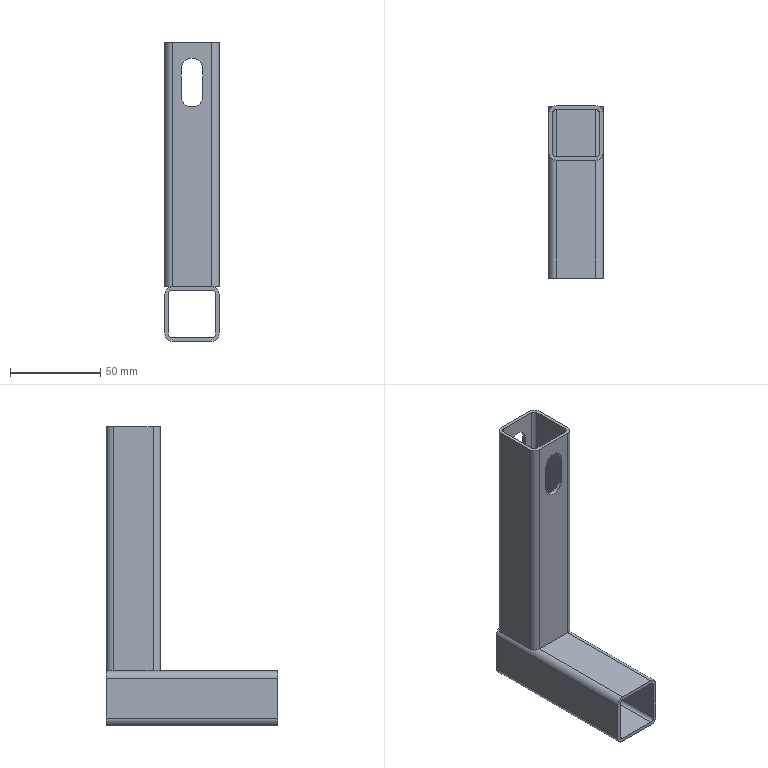Part | SolidWorks | features ICE 1, WeldMemberFeat 1, WeldmentFeature 1 | 2 solids | 46 faces | box 30 x 95 x 165 mm | volume 47978 mm3 | plane 24 | cylinder 22 | commonest cylinder face diameters 4 x8 8 x8 12 x6
STEP:
#1=CARTESIAN_POINT('',(11.,95.,15.));
#2=VERTEX_POINT('',#1);
#3=CARTESIAN_POINT('',(15.,95.,11.));
#4=VERTEX_POINT('',#3);
#5=CARTESIAN_POINT('',(11.,95.,11.));
#6=DIRECTION('',(0.,1.,0.));
#7=DIRECTION('',(0.,0.,1.));
#8=AXIS2_PLACEMENT_3D('',#5,#6,#7);
#9=CIRCLE('',#8,4.);
#10=EDGE_CURVE('',#2,#4,#9,.T.);
#11=ORIENTED_EDGE('',*,*,#10,.F.);
#12=CARTESIAN_POINT('',(11.,0.,15.));
#13=VERTEX_POINT('',#12);
#14=CARTESIAN_POINT('',(11.,80.,15.));
#15=DIRECTION('',(0.,-1.,0.));
#16=VECTOR('',#15,1000.);
#17=LINE('',#14,#16);
#18=EDGE_CURVE('',#2,#13,#17,.T.);
#19=ORIENTED_EDGE('',*,*,#18,.T.);
#20=CARTESIAN_POINT('',(15.,0.,11.));
#21=VERTEX_POINT('',#20);
#22=CARTESIAN_POINT('',(11.,0.,11.));
#23=DIRECTION('',(0.,1.,0.));
#24=DIRECTION('',(0.,0.,1.));
#25=AXIS2_PLACEMENT_3D('',#22,#23,#24);
#26=CIRCLE('',#25,4.);
#27=EDGE_CURVE('',#13,#21,#26,.T.);
#28=ORIENTED_EDGE('',*,*,#27,.T.);
#29=CARTESIAN_POINT('',(15.,80.,11.));
#30=DIRECTION('',(0.,-1.,0.));
#31=VECTOR('',#30,1000.);
#32=LINE('',#29,#31);
#33=EDGE_CURVE('',#4,#21,#32,.T.);
#34=ORIENTED_EDGE('',*,*,#33,.F.);
#35=EDGE_LOOP('',(#11,#19,#28,#34));
#36=FACE_OUTER_BOUND('',#35,.T.);
#37=CARTESIAN_POINT('',(11.,80.,11.));
#38=DIRECTION('',(0.,-1.,0.));
#39=DIRECTION('',(0.,0.,-1.));
#40=AXIS2_PLACEMENT_3D('',#37,#38,#39);
#41=CYLINDRICAL_SURFACE('',#40,4.);
#42=ADVANCED_FACE('',(#36),#41,.T.);
#43=CARTESIAN_POINT('',(15.,95.,-11.));
#44=VERTEX_POINT('',#43);
#45=CARTESIAN_POINT('',(15.,95.,11.));
#46=DIRECTION('',(0.,0.,-1.));
#47=VECTOR('',#46,1000.);
#48=LINE('',#45,#47);
#49=EDGE_CURVE('',#4,#44,#48,.T.);
#50=ORIENTED_EDGE('',*,*,#49,.F.);
#51=ORIENTED_EDGE('',*,*,#33,.T.);
#52=CARTESIAN_POINT('',(15.,0.,-11.));
#53=VERTEX_POINT('',#52);
#54=CARTESIAN_POINT('',(15.,0.,11.));
#55=DIRECTION('',(0.,0.,-1.));
#56=VECTOR('',#55,1000.);
#57=LINE('',#54,#56);
#58=EDGE_CURVE('',#21,#53,#57,.T.);
#59=ORIENTED_EDGE('',*,*,#58,.T.);
#60=CARTESIAN_POINT('',(15.,80.,-11.));
#61=DIRECTION('',(0.,-1.,0.));
#62=VECTOR('',#61,1000.);
#63=LINE('',#60,#62);
#64=EDGE_CURVE('',#44,#53,#63,.T.);
#65=ORIENTED_EDGE('',*,*,#64,.F.);
#66=EDGE_LOOP('',(#50,#51,#59,#65));
#67=FACE_OUTER_BOUND('',#66,.T.);
#68=CARTESIAN_POINT('',(15.,80.,11.));
#69=DIRECTION('',(-1.,0.,0.));
#70=DIRECTION('',(0.,0.,1.));
#71=AXIS2_PLACEMENT_3D('',#68,#69,#70);
#72=PLANE('',#71);
#73=ADVANCED_FACE('',(#67),#72,.F.);
#74=CARTESIAN_POINT('',(11.,95.,-15.));
#75=VERTEX_POINT('',#74);
#76=CARTESIAN_POINT('',(11.,95.,-11.));
#77=DIRECTION('',(0.,1.,0.));
#78=DIRECTION('',(0.,0.,1.));
#79=AXIS2_PLACEMENT_3D('',#76,#77,#78);
#80=CIRCLE('',#79,4.);
#81=EDGE_CURVE('',#44,#75,#80,.T.);
#82=ORIENTED_EDGE('',*,*,#81,.F.);
#83=ORIENTED_EDGE('',*,*,#64,.T.);
#84=CARTESIAN_POINT('',(11.,0.,-15.));
#85=VERTEX_POINT('',#84);
#86=CARTESIAN_POINT('',(11.,0.,-11.));
#87=DIRECTION('',(0.,1.,0.));
#88=DIRECTION('',(0.,0.,1.));
#89=AXIS2_PLACEMENT_3D('',#86,#87,#88);
#90=CIRCLE('',#89,4.);
#91=EDGE_CURVE('',#53,#85,#90,.T.);
#92=ORIENTED_EDGE('',*,*,#91,.T.);
#93=CARTESIAN_POINT('',(11.,80.,-15.));
#94=DIRECTION('',(0.,-1.,0.));
#95=VECTOR('',#94,1000.);
#96=LINE('',#93,#95);
#97=EDGE_CURVE('',#75,#85,#96,.T.);
#98=ORIENTED_EDGE('',*,*,#97,.F.);
#99=EDGE_LOOP('',(#82,#83,#92,#98));
#100=FACE_OUTER_BOUND('',#99,.T.);
#101=CARTESIAN_POINT('',(11.,80.,-11.));
#102=DIRECTION('',(0.,-1.,0.));
#103=DIRECTION('',(0.,0.,-1.));
#104=AXIS2_PLACEMENT_3D('',#101,#102,#103);
#105=CYLINDRICAL_SURFACE('',#104,4.);
#106=ADVANCED_FACE('',(#100),#105,.T.);
#107=CARTESIAN_POINT('',(-11.,95.,-15.));
#108=VERTEX_POINT('',#107);
#109=CARTESIAN_POINT('',(-11.,95.,-15.));
#110=DIRECTION('',(-1.,0.,0.));
#111=VECTOR('',#110,1000.);
#112=LINE('',#109,#111);
#113=EDGE_CURVE('',#75,#108,#112,.T.);
#114=ORIENTED_EDGE('',*,*,#113,.F.);
#115=ORIENTED_EDGE('',*,*,#97,.T.);
#116=CARTESIAN_POINT('',(-11.,0.,-15.));
#117=VERTEX_POINT('',#116);
#118=CARTESIAN_POINT('',(-11.,0.,-15.));
#119=DIRECTION('',(-1.,0.,0.));
#120=VECTOR('',#119,1000.);
#121=LINE('',#118,#120);
#122=EDGE_CURVE('',#85,#117,#121,.T.);
#123=ORIENTED_EDGE('',*,*,#122,.T.);
#124=CARTESIAN_POINT('',(-11.,80.,-15.));
#125=DIRECTION('',(0.,-1.,0.));
#126=VECTOR('',#125,1000.);
#127=LINE('',#124,#126);
#128=EDGE_CURVE('',#108,#117,#127,.T.);
#129=ORIENTED_EDGE('',*,*,#128,.F.);
#130=EDGE_LOOP('',(#114,#115,#123,#129));
#131=FACE_OUTER_BOUND('',#130,.T.);
#132=CARTESIAN_POINT('',(-11.,80.,-15.));
#133=DIRECTION('',(0.,0.,1.));
#134=DIRECTION('',(1.,0.,0.));
#135=AXIS2_PLACEMENT_3D('',#132,#133,#134);
#136=PLANE('',#135);
#137=ADVANCED_FACE('',(#131),#136,.F.);
#138=CARTESIAN_POINT('',(-15.,95.,-11.));
#139=VERTEX_POINT('',#138);
#140=CARTESIAN_POINT('',(-11.,95.,-11.));
#141=DIRECTION('',(0.,1.,0.));
#142=DIRECTION('',(0.,0.,1.));
#143=AXIS2_PLACEMENT_3D('',#140,#141,#142);
#144=CIRCLE('',#143,4.);
#145=EDGE_CURVE('',#108,#139,#144,.T.);
#146=ORIENTED_EDGE('',*,*,#145,.F.);
#147=ORIENTED_EDGE('',*,*,#128,.T.);
#148=CARTESIAN_POINT('',(-15.,0.,-11.));
#149=VERTEX_POINT('',#148);
#150=CARTESIAN_POINT('',(-11.,0.,-11.));
#151=DIRECTION('',(0.,1.,0.));
#152=DIRECTION('',(0.,0.,1.));
#153=AXIS2_PLACEMENT_3D('',#150,#151,#152);
#154=CIRCLE('',#153,4.);
#155=EDGE_CURVE('',#117,#149,#154,.T.);
#156=ORIENTED_EDGE('',*,*,#155,.T.);
#157=CARTESIAN_POINT('',(-15.,80.,-11.));
#158=DIRECTION('',(0.,-1.,0.));
#159=VECTOR('',#158,1000.);
#160=LINE('',#157,#159);
#161=EDGE_CURVE('',#139,#149,#160,.T.);
#162=ORIENTED_EDGE('',*,*,#161,.F.);
#163=EDGE_LOOP('',(#146,#147,#156,#162));
#164=FACE_OUTER_BOUND('',#163,.T.);
#165=CARTESIAN_POINT('',(-11.,80.,-11.));
#166=DIRECTION('',(0.,-1.,0.));
#167=DIRECTION('',(0.,0.,-1.));
#168=AXIS2_PLACEMENT_3D('',#165,#166,#167);
#169=CYLINDRICAL_SURFACE('',#168,4.);
#170=ADVANCED_FACE('',(#164),#169,.T.);
#171=CARTESIAN_POINT('',(-15.,95.,11.));
#172=VERTEX_POINT('',#171);
#173=CARTESIAN_POINT('',(-15.,95.,-11.));
#174=DIRECTION('',(0.,0.,1.));
#175=VECTOR('',#174,1000.);
#176=LINE('',#173,#175);
#177=EDGE_CURVE('',#139,#172,#176,.T.);
#178=ORIENTED_EDGE('',*,*,#177,.F.);
#179=ORIENTED_EDGE('',*,*,#161,.T.);
#180=CARTESIAN_POINT('',(-15.,0.,11.));
#181=VERTEX_POINT('',#180);
#182=CARTESIAN_POINT('',(-15.,0.,-11.));
#183=DIRECTION('',(0.,0.,1.));
#184=VECTOR('',#183,1000.);
#185=LINE('',#182,#184);
#186=EDGE_CURVE('',#149,#181,#185,.T.);
#187=ORIENTED_EDGE('',*,*,#186,.T.);
#188=CARTESIAN_POINT('',(-15.,80.,11.));
#189=DIRECTION('',(0.,-1.,0.));
#190=VECTOR('',#189,1000.);
#191=LINE('',#188,#190);
#192=EDGE_CURVE('',#172,#181,#191,.T.);
#193=ORIENTED_EDGE('',*,*,#192,.F.);
#194=EDGE_LOOP('',(#178,#179,#187,#193));
#195=FACE_OUTER_BOUND('',#194,.T.);
#196=CARTESIAN_POINT('',(-15.,80.,-11.));
#197=DIRECTION('',(1.,0.,0.));
#198=DIRECTION('',(0.,0.,-1.));
#199=AXIS2_PLACEMENT_3D('',#196,#197,#198);
#200=PLANE('',#199);
#201=ADVANCED_FACE('',(#195),#200,.F.);
#202=CARTESIAN_POINT('',(-11.,95.,15.));
#203=VERTEX_POINT('',#202);
#204=CARTESIAN_POINT('',(-11.,95.,11.));
#205=DIRECTION('',(0.,1.,0.));
#206=DIRECTION('',(0.,0.,1.));
#207=AXIS2_PLACEMENT_3D('',#204,#205,#206);
#208=CIRCLE('',#207,4.);
#209=EDGE_CURVE('',#172,#203,#208,.T.);
#210=ORIENTED_EDGE('',*,*,#209,.F.);
#211=ORIENTED_EDGE('',*,*,#192,.T.);
#212=CARTESIAN_POINT('',(-11.,0.,15.));
#213=VERTEX_POINT('',#212);
#214=CARTESIAN_POINT('',(-11.,0.,11.));
#215=DIRECTION('',(0.,1.,0.));
#216=DIRECTION('',(0.,0.,1.));
#217=AXIS2_PLACEMENT_3D('',#214,#215,#216);
#218=CIRCLE('',#217,4.);
#219=EDGE_CURVE('',#181,#213,#218,.T.);
#220=ORIENTED_EDGE('',*,*,#219,.T.);
#221=CARTESIAN_POINT('',(-11.,80.,15.));
#222=DIRECTION('',(0.,-1.,0.));
#223=VECTOR('',#222,1000.);
#224=LINE('',#221,#223);
#225=EDGE_CURVE('',#203,#213,#224,.T.);
#226=ORIENTED_EDGE('',*,*,#225,.F.);
#227=EDGE_LOOP('',(#210,#211,#220,#226));
#228=FACE_OUTER_BOUND('',#227,.T.);
#229=CARTESIAN_POINT('',(-11.,80.,11.));
#230=DIRECTION('',(0.,-1.,0.));
#231=DIRECTION('',(0.,0.,-1.));
#232=AXIS2_PLACEMENT_3D('',#229,#230,#231);
#233=CYLINDRICAL_SURFACE('',#232,4.);
#234=ADVANCED_FACE('',(#228),#233,.T.);
#235=CARTESIAN_POINT('',(13.,95.,-11.));
#236=VERTEX_POINT('',#235);
#237=CARTESIAN_POINT('',(13.,0.,-11.));
#238=VERTEX_POINT('',#237);
#239=CARTESIAN_POINT('',(13.,80.,-11.));
#240=DIRECTION('',(0.,-1.,0.));
#241=VECTOR('',#240,1000.);
#242=LINE('',#239,#241);
#243=EDGE_CURVE('',#236,#238,#242,.T.);
#244=ORIENTED_EDGE('',*,*,#243,.F.);
#245=CARTESIAN_POINT('',(11.,95.,-13.));
#246=VERTEX_POINT('',#245);
#247=CARTESIAN_POINT('',(11.,95.,-11.));
#248=DIRECTION('',(0.,1.,0.));
#249=DIRECTION('',(0.,0.,1.));
#250=AXIS2_PLACEMENT_3D('',#247,#248,#249);
#251=CIRCLE('',#250,2.);
#252=EDGE_CURVE('',#236,#246,#251,.T.);
#253=ORIENTED_EDGE('',*,*,#252,.T.);
#254=CARTESIAN_POINT('',(11.,0.,-13.));
#255=VERTEX_POINT('',#254);
#256=CARTESIAN_POINT('',(11.,80.,-13.));
#257=DIRECTION('',(0.,-1.,0.));
#258=VECTOR('',#257,1000.);
#259=LINE('',#256,#258);
#260=EDGE_CURVE('',#246,#255,#259,.T.);
#261=ORIENTED_EDGE('',*,*,#260,.T.);
#262=CARTESIAN_POINT('',(11.,0.,-11.));
#263=DIRECTION('',(0.,1.,0.));
#264=DIRECTION('',(0.,0.,1.));
#265=AXIS2_PLACEMENT_3D('',#262,#263,#264);
#266=CIRCLE('',#265,2.);
#267=EDGE_CURVE('',#238,#255,#266,.T.);
#268=ORIENTED_EDGE('',*,*,#267,.F.);
#269=EDGE_LOOP('',(#244,#253,#261,#268));
#270=FACE_OUTER_BOUND('',#269,.T.);
#271=CARTESIAN_POINT('',(11.,80.,-11.));
#272=DIRECTION('',(0.,-1.,0.));
#273=DIRECTION('',(0.,0.,-1.));
#274=AXIS2_PLACEMENT_3D('',#271,#272,#273);
#275=CYLINDRICAL_SURFACE('',#274,2.);
#276=ADVANCED_FACE('',(#270),#275,.F.);
#277=CARTESIAN_POINT('',(13.,95.,11.));
#278=VERTEX_POINT('',#277);
#279=CARTESIAN_POINT('',(13.,0.,11.));
#280=VERTEX_POINT('',#279);
#281=CARTESIAN_POINT('',(13.,80.,11.));
#282=DIRECTION('',(0.,-1.,0.));
#283=VECTOR('',#282,1000.);
#284=LINE('',#281,#283);
#285=EDGE_CURVE('',#278,#280,#284,.T.);
#286=ORIENTED_EDGE('',*,*,#285,.F.);
#287=CARTESIAN_POINT('',(13.,95.,11.));
#288=DIRECTION('',(0.,0.,-1.));
#289=VECTOR('',#288,1000.);
#290=LINE('',#287,#289);
#291=EDGE_CURVE('',#278,#236,#290,.T.);
#292=ORIENTED_EDGE('',*,*,#291,.T.);
#293=ORIENTED_EDGE('',*,*,#243,.T.);
#294=CARTESIAN_POINT('',(13.,0.,11.));
#295=DIRECTION('',(0.,0.,-1.));
#296=VECTOR('',#295,1000.);
#297=LINE('',#294,#296);
#298=EDGE_CURVE('',#280,#238,#297,.T.);
#299=ORIENTED_EDGE('',*,*,#298,.F.);
#300=EDGE_LOOP('',(#286,#292,#293,#299));
#301=FACE_OUTER_BOUND('',#300,.T.);
#302=CARTESIAN_POINT('',(13.,80.,11.));
#303=DIRECTION('',(-1.,0.,0.));
#304=DIRECTION('',(0.,0.,1.));
#305=AXIS2_PLACEMENT_3D('',#302,#303,#304);
#306=PLANE('',#305);
#307=ADVANCED_FACE('',(#301),#306,.T.);
#308=CARTESIAN_POINT('',(11.,95.,13.));
#309=VERTEX_POINT('',#308);
#310=CARTESIAN_POINT('',(11.,0.,13.));
#311=VERTEX_POINT('',#310);
#312=CARTESIAN_POINT('',(11.,80.,13.));
#313=DIRECTION('',(0.,-1.,0.));
#314=VECTOR('',#313,1000.);
#315=LINE('',#312,#314);
#316=EDGE_CURVE('',#309,#311,#315,.T.);
#317=ORIENTED_EDGE('',*,*,#316,.F.);
#318=CARTESIAN_POINT('',(11.,95.,11.));
#319=DIRECTION('',(0.,1.,0.));
#320=DIRECTION('',(0.,0.,1.));
#321=AXIS2_PLACEMENT_3D('',#318,#319,#320);
#322=CIRCLE('',#321,2.);
#323=EDGE_CURVE('',#309,#278,#322,.T.);
#324=ORIENTED_EDGE('',*,*,#323,.T.);
#325=ORIENTED_EDGE('',*,*,#285,.T.);
#326=CARTESIAN_POINT('',(11.,0.,11.));
#327=DIRECTION('',(0.,1.,0.));
#328=DIRECTION('',(0.,0.,1.));
#329=AXIS2_PLACEMENT_3D('',#326,#327,#328);
#330=CIRCLE('',#329,2.);
#331=EDGE_CURVE('',#311,#280,#330,.T.);
#332=ORIENTED_EDGE('',*,*,#331,.F.);
#333=EDGE_LOOP('',(#317,#324,#325,#332));
#334=FACE_OUTER_BOUND('',#333,.T.);
#335=CARTESIAN_POINT('',(11.,80.,11.));
#336=DIRECTION('',(0.,-1.,0.));
#337=DIRECTION('',(0.,0.,-1.));
#338=AXIS2_PLACEMENT_3D('',#335,#336,#337);
#339=CYLINDRICAL_SURFACE('',#338,2.);
#340=ADVANCED_FACE('',(#334),#339,.F.);
#341=CARTESIAN_POINT('',(-11.,95.,13.));
#342=VERTEX_POINT('',#341);
#343=CARTESIAN_POINT('',(-11.,0.,13.));
#344=VERTEX_POINT('',#343);
#345=CARTESIAN_POINT('',(-11.,80.,13.));
#346=DIRECTION('',(0.,-1.,0.));
#347=VECTOR('',#346,1000.);
#348=LINE('',#345,#347);
#349=EDGE_CURVE('',#342,#344,#348,.T.);
#350=ORIENTED_EDGE('',*,*,#349,.F.);
#351=CARTESIAN_POINT('',(11.,95.,13.));
#352=DIRECTION('',(1.,0.,0.));
#353=VECTOR('',#352,1000.);
#354=LINE('',#351,#353);
#355=EDGE_CURVE('',#342,#309,#354,.T.);
#356=ORIENTED_EDGE('',*,*,#355,.T.);
#357=ORIENTED_EDGE('',*,*,#316,.T.);
#358=CARTESIAN_POINT('',(11.,0.,13.));
#359=DIRECTION('',(1.,0.,0.));
#360=VECTOR('',#359,1000.);
#361=LINE('',#358,#360);
#362=EDGE_CURVE('',#344,#311,#361,.T.);
#363=ORIENTED_EDGE('',*,*,#362,.F.);
#364=EDGE_LOOP('',(#350,#356,#357,#363));
#365=FACE_OUTER_BOUND('',#364,.T.);
#366=CARTESIAN_POINT('',(11.,80.,13.));
#367=DIRECTION('',(0.,0.,-1.));
#368=DIRECTION('',(-1.,0.,0.));
#369=AXIS2_PLACEMENT_3D('',#366,#367,#368);
#370=PLANE('',#369);
#371=ADVANCED_FACE('',(#365),#370,.T.);
#372=CARTESIAN_POINT('',(-13.,95.,11.));
#373=VERTEX_POINT('',#372);
#374=CARTESIAN_POINT('',(-13.,0.,11.));
#375=VERTEX_POINT('',#374);
#376=CARTESIAN_POINT('',(-13.,80.,11.));
#377=DIRECTION('',(0.,-1.,0.));
#378=VECTOR('',#377,1000.);
#379=LINE('',#376,#378);
#380=EDGE_CURVE('',#373,#375,#379,.T.);
#381=ORIENTED_EDGE('',*,*,#380,.F.);
#382=CARTESIAN_POINT('',(-11.,95.,11.));
#383=DIRECTION('',(0.,1.,0.));
#384=DIRECTION('',(0.,0.,1.));
#385=AXIS2_PLACEMENT_3D('',#382,#383,#384);
#386=CIRCLE('',#385,2.);
#387=EDGE_CURVE('',#373,#342,#386,.T.);
#388=ORIENTED_EDGE('',*,*,#387,.T.);
#389=ORIENTED_EDGE('',*,*,#349,.T.);
#390=CARTESIAN_POINT('',(-11.,0.,11.));
#391=DIRECTION('',(0.,1.,0.));
#392=DIRECTION('',(0.,0.,1.));
#393=AXIS2_PLACEMENT_3D('',#390,#391,#392);
#394=CIRCLE('',#393,2.);
#395=EDGE_CURVE('',#375,#344,#394,.T.);
#396=ORIENTED_EDGE('',*,*,#395,.F.);
#397=EDGE_LOOP('',(#381,#388,#389,#396));
#398=FACE_OUTER_BOUND('',#397,.T.);
#399=CARTESIAN_POINT('',(-11.,80.,11.));
#400=DIRECTION('',(0.,-1.,0.));
#401=DIRECTION('',(0.,0.,-1.));
#402=AXIS2_PLACEMENT_3D('',#399,#400,#401);
#403=CYLINDRICAL_SURFACE('',#402,2.);
#404=ADVANCED_FACE('',(#398),#403,.F.);
#405=CARTESIAN_POINT('',(-13.,95.,-11.));
#406=VERTEX_POINT('',#405);
#407=CARTESIAN_POINT('',(-13.,0.,-11.));
#408=VERTEX_POINT('',#407);
#409=CARTESIAN_POINT('',(-13.,80.,-11.));
#410=DIRECTION('',(0.,-1.,0.));
#411=VECTOR('',#410,1000.);
#412=LINE('',#409,#411);
#413=EDGE_CURVE('',#406,#408,#412,.T.);
#414=ORIENTED_EDGE('',*,*,#413,.F.);
#415=CARTESIAN_POINT('',(-13.,95.,-11.));
#416=DIRECTION('',(0.,0.,1.));
#417=VECTOR('',#416,1000.);
#418=LINE('',#415,#417);
#419=EDGE_CURVE('',#406,#373,#418,.T.);
#420=ORIENTED_EDGE('',*,*,#419,.T.);
#421=ORIENTED_EDGE('',*,*,#380,.T.);
#422=CARTESIAN_POINT('',(-13.,0.,-11.));
#423=DIRECTION('',(0.,0.,1.));
#424=VECTOR('',#423,1000.);
#425=LINE('',#422,#424);
#426=EDGE_CURVE('',#408,#375,#425,.T.);
#427=ORIENTED_EDGE('',*,*,#426,.F.);
#428=EDGE_LOOP('',(#414,#420,#421,#427));
#429=FACE_OUTER_BOUND('',#428,.T.);
#430=CARTESIAN_POINT('',(-13.,80.,-11.));
#431=DIRECTION('',(1.,0.,0.));
#432=DIRECTION('',(0.,0.,-1.));
#433=AXIS2_PLACEMENT_3D('',#430,#431,#432);
#434=PLANE('',#433);
#435=ADVANCED_FACE('',(#429),#434,.T.);
#436=CARTESIAN_POINT('',(-11.,95.,-13.));
#437=VERTEX_POINT('',#436);
#438=CARTESIAN_POINT('',(-11.,0.,-13.));
#439=VERTEX_POINT('',#438);
#440=CARTESIAN_POINT('',(-11.,80.,-13.));
#441=DIRECTION('',(0.,-1.,0.));
#442=VECTOR('',#441,1000.);
#443=LINE('',#440,#442);
#444=EDGE_CURVE('',#437,#439,#443,.T.);
#445=ORIENTED_EDGE('',*,*,#444,.F.);
#446=CARTESIAN_POINT('',(-11.,95.,-11.));
#447=DIRECTION('',(0.,1.,0.));
#448=DIRECTION('',(0.,0.,1.));
#449=AXIS2_PLACEMENT_3D('',#446,#447,#448);
#450=CIRCLE('',#449,2.);
#451=EDGE_CURVE('',#437,#406,#450,.T.);
#452=ORIENTED_EDGE('',*,*,#451,.T.);
#453=ORIENTED_EDGE('',*,*,#413,.T.);
#454=CARTESIAN_POINT('',(-11.,0.,-11.));
#455=DIRECTION('',(0.,1.,0.));
#456=DIRECTION('',(0.,0.,1.));
#457=AXIS2_PLACEMENT_3D('',#454,#455,#456);
#458=CIRCLE('',#457,2.);
#459=EDGE_CURVE('',#439,#408,#458,.T.);
#460=ORIENTED_EDGE('',*,*,#459,.F.);
#461=EDGE_LOOP('',(#445,#452,#453,#460));
#462=FACE_OUTER_BOUND('',#461,.T.);
#463=CARTESIAN_POINT('',(-11.,80.,-11.));
#464=DIRECTION('',(0.,-1.,0.));
#465=DIRECTION('',(0.,0.,-1.));
#466=AXIS2_PLACEMENT_3D('',#463,#464,#465);
#467=CYLINDRICAL_SURFACE('',#466,2.);
#468=ADVANCED_FACE('',(#462),#467,.F.);
#469=ORIENTED_EDGE('',*,*,#260,.F.);
#470=CARTESIAN_POINT('',(-11.,95.,-13.));
#471=DIRECTION('',(-1.,0.,0.));
#472=VECTOR('',#471,1000.);
#473=LINE('',#470,#472);
#474=EDGE_CURVE('',#246,#437,#473,.T.);
#475=ORIENTED_EDGE('',*,*,#474,.T.);
#476=ORIENTED_EDGE('',*,*,#444,.T.);
#477=CARTESIAN_POINT('',(-11.,0.,-13.));
#478=DIRECTION('',(-1.,0.,0.));
#479=VECTOR('',#478,1000.);
#480=LINE('',#477,#479);
#481=EDGE_CURVE('',#255,#439,#480,.T.);
#482=ORIENTED_EDGE('',*,*,#481,.F.);
#483=EDGE_LOOP('',(#469,#475,#476,#482));
#484=FACE_OUTER_BOUND('',#483,.T.);
#485=CARTESIAN_POINT('',(-11.,80.,-13.));
#486=DIRECTION('',(0.,0.,1.));
#487=DIRECTION('',(1.,0.,0.));
#488=AXIS2_PLACEMENT_3D('',#485,#486,#487);
#489=PLANE('',#488);
#490=ADVANCED_FACE('',(#484),#489,.T.);
#491=CARTESIAN_POINT('',(11.,95.,15.));
#492=DIRECTION('',(1.,0.,0.));
#493=VECTOR('',#492,1000.);
#494=LINE('',#491,#493);
#495=EDGE_CURVE('',#203,#2,#494,.T.);
#496=ORIENTED_EDGE('',*,*,#495,.F.);
#497=ORIENTED_EDGE('',*,*,#225,.T.);
#498=CARTESIAN_POINT('',(11.,0.,15.));
#499=DIRECTION('',(1.,0.,0.));
#500=VECTOR('',#499,1000.);
#501=LINE('',#498,#500);
#502=EDGE_CURVE('',#213,#13,#501,.T.);
#503=ORIENTED_EDGE('',*,*,#502,.T.);
#504=ORIENTED_EDGE('',*,*,#18,.F.);
#505=EDGE_LOOP('',(#496,#497,#503,#504));
#506=FACE_OUTER_BOUND('',#505,.T.);
#507=CARTESIAN_POINT('',(11.,80.,15.));
#508=DIRECTION('',(0.,0.,-1.));
#509=DIRECTION('',(-1.,0.,0.));
#510=AXIS2_PLACEMENT_3D('',#507,#508,#509);
#511=PLANE('',#510);
#512=ADVANCED_FACE('',(#506),#511,.F.);
#513=ORIENTED_EDGE('',*,*,#267,.T.);
#514=ORIENTED_EDGE('',*,*,#481,.T.);
#515=ORIENTED_EDGE('',*,*,#459,.T.);
#516=ORIENTED_EDGE('',*,*,#426,.T.);
#517=ORIENTED_EDGE('',*,*,#395,.T.);
#518=ORIENTED_EDGE('',*,*,#362,.T.);
#519=ORIENTED_EDGE('',*,*,#331,.T.);
#520=ORIENTED_EDGE('',*,*,#298,.T.);
#521=EDGE_LOOP('',(#513,#514,#515,#516,#517,#518,#519,#520));
#522=FACE_BOUND('',#521,.T.);
#523=ORIENTED_EDGE('',*,*,#27,.F.);
#524=ORIENTED_EDGE('',*,*,#502,.F.);
#525=ORIENTED_EDGE('',*,*,#219,.F.);
#526=ORIENTED_EDGE('',*,*,#186,.F.);
#527=ORIENTED_EDGE('',*,*,#155,.F.);
#528=ORIENTED_EDGE('',*,*,#122,.F.);
#529=ORIENTED_EDGE('',*,*,#91,.F.);
#530=ORIENTED_EDGE('',*,*,#58,.F.);
#531=EDGE_LOOP('',(#523,#524,#525,#526,#527,#528,#529,#530));
#532=FACE_OUTER_BOUND('',#531,.T.);
#533=CARTESIAN_POINT('',(11.,0.,11.));
#534=DIRECTION('',(0.,1.,0.));
#535=DIRECTION('',(0.,0.,1.));
#536=AXIS2_PLACEMENT_3D('',#533,#534,#535);
#537=PLANE('',#536);
#538=ADVANCED_FACE('',(#522,#532),#537,.F.);
#539=ORIENTED_EDGE('',*,*,#252,.F.);
#540=ORIENTED_EDGE('',*,*,#291,.F.);
#541=ORIENTED_EDGE('',*,*,#323,.F.);
#542=ORIENTED_EDGE('',*,*,#355,.F.);
#543=ORIENTED_EDGE('',*,*,#387,.F.);
#544=ORIENTED_EDGE('',*,*,#419,.F.);
#545=ORIENTED_EDGE('',*,*,#451,.F.);
#546=ORIENTED_EDGE('',*,*,#474,.F.);
#547=EDGE_LOOP('',(#539,#540,#541,#542,#543,#544,#545,#546));
#548=FACE_BOUND('',#547,.T.);
#549=ORIENTED_EDGE('',*,*,#495,.T.);
#550=ORIENTED_EDGE('',*,*,#10,.T.);
#551=ORIENTED_EDGE('',*,*,#49,.T.);
#552=ORIENTED_EDGE('',*,*,#81,.T.);
#553=ORIENTED_EDGE('',*,*,#113,.T.);
#554=ORIENTED_EDGE('',*,*,#145,.T.);
#555=ORIENTED_EDGE('',*,*,#177,.T.);
#556=ORIENTED_EDGE('',*,*,#209,.T.);
#557=EDGE_LOOP('',(#549,#550,#551,#552,#553,#554,#555,#556));
#558=FACE_OUTER_BOUND('',#557,.T.);
#559=CARTESIAN_POINT('',(15.,95.,0.));
#560=DIRECTION('',(0.,1.,0.));
#561=DIRECTION('',(0.,0.,1.));
#562=AXIS2_PLACEMENT_3D('',#559,#560,#561);
#563=PLANE('',#562);
#564=ADVANCED_FACE('',(#548,#558),#563,.T.);
#565=CLOSED_SHELL('',(#42,#73,#106,#137,#170,#201,#234,#276,#307,#340,#371,#404,#435,#468,#490,#512,#538,#564));
#566=MANIFOLD_SOLID_BREP('',#565);
#567=CARTESIAN_POINT('',(6.,93.,135.514));
#568=VERTEX_POINT('',#567);
#569=CARTESIAN_POINT('',(0.,93.,141.514));
#570=VERTEX_POINT('',#569);
#571=CARTESIAN_POINT('',(0.,93.,135.514));
#572=DIRECTION('',(0.,-1.,0.));
#573=DIRECTION('',(0.,0.,-1.));
#574=AXIS2_PLACEMENT_3D('',#571,#572,#573);
#575=CIRCLE('',#574,6.);
#576=EDGE_CURVE('',#568,#570,#575,.T.);
#577=ORIENTED_EDGE('',*,*,#576,.T.);
#578=CARTESIAN_POINT('',(0.,95.,141.514));
#579=VERTEX_POINT('',#578);
#580=CARTESIAN_POINT('',(0.,28.,141.514));
#581=DIRECTION('',(0.,1.,0.));
#582=VECTOR('',#581,1000.);
#583=LINE('',#580,#582);
#584=EDGE_CURVE('',#570,#579,#583,.T.);
#585=ORIENTED_EDGE('',*,*,#584,.T.);
#586=CARTESIAN_POINT('',(6.,95.,135.514));
#587=VERTEX_POINT('',#586);
#588=CARTESIAN_POINT('',(0.,95.,135.514));
#589=DIRECTION('',(0.,1.,0.));
#590=DIRECTION('',(0.,0.,1.));
#591=AXIS2_PLACEMENT_3D('',#588,#589,#590);
#592=CIRCLE('',#591,6.);
#593=EDGE_CURVE('',#579,#587,#592,.T.);
#594=ORIENTED_EDGE('',*,*,#593,.T.);
#595=CARTESIAN_POINT('',(6.,28.,135.514));
#596=DIRECTION('',(0.,1.,0.));
#597=VECTOR('',#596,1000.);
#598=LINE('',#595,#597);
#599=EDGE_CURVE('',#568,#587,#598,.T.);
#600=ORIENTED_EDGE('',*,*,#599,.F.);
#601=EDGE_LOOP('',(#577,#585,#594,#600));
#602=FACE_OUTER_BOUND('',#601,.T.);
#603=CARTESIAN_POINT('',(0.,28.,135.514));
#604=DIRECTION('',(0.,1.,0.));
#605=DIRECTION('',(0.,0.,1.));
#606=AXIS2_PLACEMENT_3D('',#603,#604,#605);
#607=CYLINDRICAL_SURFACE('',#606,6.);
#608=ADVANCED_FACE('',(#602),#607,.F.);
#609=CARTESIAN_POINT('',(0.,65.,141.514));
#610=VERTEX_POINT('',#609);
#611=CARTESIAN_POINT('',(6.,65.,135.514));
#612=VERTEX_POINT('',#611);
#613=CARTESIAN_POINT('',(0.,65.,135.514));
#614=DIRECTION('',(0.,1.,0.));
#615=DIRECTION('',(0.,0.,1.));
#616=AXIS2_PLACEMENT_3D('',#613,#614,#615);
#617=CIRCLE('',#616,6.);
#618=EDGE_CURVE('',#610,#612,#617,.T.);
#619=ORIENTED_EDGE('',*,*,#618,.F.);
#620=CARTESIAN_POINT('',(0.,67.,141.514));
#621=VERTEX_POINT('',#620);
#622=CARTESIAN_POINT('',(0.,28.,141.514));
#623=DIRECTION('',(0.,1.,0.));
#624=VECTOR('',#623,1000.);
#625=LINE('',#622,#624);
#626=EDGE_CURVE('',#610,#621,#625,.T.);
#627=ORIENTED_EDGE('',*,*,#626,.T.);
#628=CARTESIAN_POINT('',(6.,67.,135.514));
#629=VERTEX_POINT('',#628);
#630=CARTESIAN_POINT('',(0.,67.,135.514));
#631=DIRECTION('',(0.,1.,0.));
#632=DIRECTION('',(0.,0.,1.));
#633=AXIS2_PLACEMENT_3D('',#630,#631,#632);
#634=CIRCLE('',#633,6.);
#635=EDGE_CURVE('',#621,#629,#634,.T.);
#636=ORIENTED_EDGE('',*,*,#635,.T.);
#637=CARTESIAN_POINT('',(6.,28.,135.514));
#638=DIRECTION('',(0.,1.,0.));
#639=VECTOR('',#638,1000.);
#640=LINE('',#637,#639);
#641=EDGE_CURVE('',#612,#629,#640,.T.);
#642=ORIENTED_EDGE('',*,*,#641,.F.);
#643=EDGE_LOOP('',(#619,#627,#636,#642));
#644=FACE_OUTER_BOUND('',#643,.T.);
#645=CARTESIAN_POINT('',(0.,28.,135.514));
#646=DIRECTION('',(0.,1.,0.));
#647=DIRECTION('',(0.,0.,1.));
#648=AXIS2_PLACEMENT_3D('',#645,#646,#647);
#649=CYLINDRICAL_SURFACE('',#648,6.);
#650=ADVANCED_FACE('',(#644),#649,.F.);
#651=CARTESIAN_POINT('',(15.,69.,15.));
#652=VERTEX_POINT('',#651);
#653=CARTESIAN_POINT('',(11.,65.,15.));
#654=VERTEX_POINT('',#653);
#655=CARTESIAN_POINT('',(11.,69.,15.));
#656=DIRECTION('',(0.,0.,-1.));
#657=DIRECTION('',(-1.,0.,0.));
#658=AXIS2_PLACEMENT_3D('',#655,#656,#657);
#659=CIRCLE('',#658,4.);
#660=EDGE_CURVE('',#652,#654,#659,.T.);
#661=ORIENTED_EDGE('',*,*,#660,.F.);
#662=CARTESIAN_POINT('',(15.,69.,150.));
#663=VERTEX_POINT('',#662);
#664=CARTESIAN_POINT('',(15.,69.,150.));
#665=DIRECTION('',(0.,0.,-1.));
#666=VECTOR('',#665,1000.);
#667=LINE('',#664,#666);
#668=EDGE_CURVE('',#663,#652,#667,.T.);
#669=ORIENTED_EDGE('',*,*,#668,.F.);
#670=CARTESIAN_POINT('',(11.,65.,150.));
#671=VERTEX_POINT('',#670);
#672=CARTESIAN_POINT('',(11.,69.,150.));
#673=DIRECTION('',(0.,0.,1.));
#674=DIRECTION('',(0.,-1.,0.));
#675=AXIS2_PLACEMENT_3D('',#672,#673,#674);
#676=CIRCLE('',#675,4.);
#677=EDGE_CURVE('',#671,#663,#676,.T.);
#678=ORIENTED_EDGE('',*,*,#677,.F.);
#679=CARTESIAN_POINT('',(11.,65.,150.));
#680=DIRECTION('',(0.,0.,-1.));
#681=VECTOR('',#680,1000.);
#682=LINE('',#679,#681);
#683=EDGE_CURVE('',#671,#654,#682,.T.);
#684=ORIENTED_EDGE('',*,*,#683,.T.);
#685=EDGE_LOOP('',(#661,#669,#678,#684));
#686=FACE_OUTER_BOUND('',#685,.T.);
#687=CARTESIAN_POINT('',(11.,69.,150.));
#688=DIRECTION('',(0.,0.,-1.));
#689=DIRECTION('',(0.,1.,0.));
#690=AXIS2_PLACEMENT_3D('',#687,#688,#689);
#691=CYLINDRICAL_SURFACE('',#690,4.);
#692=ADVANCED_FACE('',(#686),#691,.T.);
#693=CARTESIAN_POINT('',(15.,91.,15.));
#694=VERTEX_POINT('',#693);
#695=CARTESIAN_POINT('',(15.,80.,15.));
#696=DIRECTION('',(0.,-1.,0.));
#697=VECTOR('',#696,1000.);
#698=LINE('',#695,#697);
#699=EDGE_CURVE('',#694,#652,#698,.T.);
#700=ORIENTED_EDGE('',*,*,#699,.F.);
#701=CARTESIAN_POINT('',(15.,91.,150.));
#702=VERTEX_POINT('',#701);
#703=CARTESIAN_POINT('',(15.,91.,150.));
#704=DIRECTION('',(0.,0.,-1.));
#705=VECTOR('',#704,1000.);
#706=LINE('',#703,#705);
#707=EDGE_CURVE('',#702,#694,#706,.T.);
#708=ORIENTED_EDGE('',*,*,#707,.F.);
#709=CARTESIAN_POINT('',(15.,69.,150.));
#710=DIRECTION('',(0.,1.,0.));
#711=VECTOR('',#710,1000.);
#712=LINE('',#709,#711);
#713=EDGE_CURVE('',#663,#702,#712,.T.);
#714=ORIENTED_EDGE('',*,*,#713,.F.);
#715=ORIENTED_EDGE('',*,*,#668,.T.);
#716=EDGE_LOOP('',(#700,#708,#714,#715));
#717=FACE_OUTER_BOUND('',#716,.T.);
#718=CARTESIAN_POINT('',(15.,69.,150.));
#719=DIRECTION('',(-1.,0.,0.));
#720=DIRECTION('',(0.,0.,1.));
#721=AXIS2_PLACEMENT_3D('',#718,#719,#720);
#722=PLANE('',#721);
#723=ADVANCED_FACE('',(#717),#722,.F.);
#724=CARTESIAN_POINT('',(11.,95.,15.));
#725=VERTEX_POINT('',#724);
#726=CARTESIAN_POINT('',(11.,91.,15.));
#727=DIRECTION('',(0.,0.,-1.));
#728=DIRECTION('',(-1.,0.,0.));
#729=AXIS2_PLACEMENT_3D('',#726,#727,#728);
#730=CIRCLE('',#729,4.);
#731=EDGE_CURVE('',#725,#694,#730,.T.);
#732=ORIENTED_EDGE('',*,*,#731,.F.);
#733=CARTESIAN_POINT('',(11.,95.,150.));
#734=VERTEX_POINT('',#733);
#735=CARTESIAN_POINT('',(11.,95.,150.));
#736=DIRECTION('',(0.,0.,-1.));
#737=VECTOR('',#736,1000.);
#738=LINE('',#735,#737);
#739=EDGE_CURVE('',#734,#725,#738,.T.);
#740=ORIENTED_EDGE('',*,*,#739,.F.);
#741=CARTESIAN_POINT('',(11.,91.,150.));
#742=DIRECTION('',(0.,0.,1.));
#743=DIRECTION('',(0.,-1.,0.));
#744=AXIS2_PLACEMENT_3D('',#741,#742,#743);
#745=CIRCLE('',#744,4.);
#746=EDGE_CURVE('',#702,#734,#745,.T.);
#747=ORIENTED_EDGE('',*,*,#746,.F.);
#748=ORIENTED_EDGE('',*,*,#707,.T.);
#749=EDGE_LOOP('',(#732,#740,#747,#748));
#750=FACE_OUTER_BOUND('',#749,.T.);
#751=CARTESIAN_POINT('',(11.,91.,150.));
#752=DIRECTION('',(0.,0.,-1.));
#753=DIRECTION('',(0.,1.,0.));
#754=AXIS2_PLACEMENT_3D('',#751,#752,#753);
#755=CYLINDRICAL_SURFACE('',#754,4.);
#756=ADVANCED_FACE('',(#750),#755,.T.);
#757=CARTESIAN_POINT('',(6.,95.,120.514));
#758=VERTEX_POINT('',#757);
#759=CARTESIAN_POINT('',(6.,95.,135.514));
#760=DIRECTION('',(0.,0.,-1.));
#761=VECTOR('',#760,1000.);
#762=LINE('',#759,#761);
#763=EDGE_CURVE('',#587,#758,#762,.T.);
#764=ORIENTED_EDGE('',*,*,#763,.F.);
#765=ORIENTED_EDGE('',*,*,#593,.F.);
#766=CARTESIAN_POINT('',(-6.,95.,135.514));
#767=VERTEX_POINT('',#766);
#768=CARTESIAN_POINT('',(0.,95.,135.514));
#769=DIRECTION('',(0.,1.,0.));
#770=DIRECTION('',(0.,0.,1.));
#771=AXIS2_PLACEMENT_3D('',#768,#769,#770);
#772=CIRCLE('',#771,6.);
#773=EDGE_CURVE('',#767,#579,#772,.T.);
#774=ORIENTED_EDGE('',*,*,#773,.F.);
#775=CARTESIAN_POINT('',(-6.,95.,120.514));
#776=VERTEX_POINT('',#775);
#777=CARTESIAN_POINT('',(-6.,95.,135.514));
#778=DIRECTION('',(0.,0.,1.));
#779=VECTOR('',#778,1000.);
#780=LINE('',#777,#779);
#781=EDGE_CURVE('',#776,#767,#780,.T.);
#782=ORIENTED_EDGE('',*,*,#781,.F.);
#783=CARTESIAN_POINT('',(0.,95.,120.514));
#784=DIRECTION('',(0.,1.,0.));
#785=DIRECTION('',(0.,0.,1.));
#786=AXIS2_PLACEMENT_3D('',#783,#784,#785);
#787=CIRCLE('',#786,6.);
#788=EDGE_CURVE('',#758,#776,#787,.T.);
#789=ORIENTED_EDGE('',*,*,#788,.F.);
#790=EDGE_LOOP('',(#764,#765,#774,#782,#789));
#791=FACE_BOUND('',#790,.T.);
#792=CARTESIAN_POINT('',(-11.,95.,15.));
#793=VERTEX_POINT('',#792);
#794=CARTESIAN_POINT('',(-11.,95.,15.));
#795=DIRECTION('',(1.,0.,0.));
#796=VECTOR('',#795,1000.);
#797=LINE('',#794,#796);
#798=EDGE_CURVE('',#793,#725,#797,.T.);
#799=ORIENTED_EDGE('',*,*,#798,.F.);
#800=CARTESIAN_POINT('',(-11.,95.,150.));
#801=VERTEX_POINT('',#800);
#802=CARTESIAN_POINT('',(-11.,95.,150.));
#803=DIRECTION('',(0.,0.,-1.));
#804=VECTOR('',#803,1000.);
#805=LINE('',#802,#804);
#806=EDGE_CURVE('',#801,#793,#805,.T.);
#807=ORIENTED_EDGE('',*,*,#806,.F.);
#808=CARTESIAN_POINT('',(-11.,95.,150.));
#809=DIRECTION('',(-1.,0.,0.));
#810=VECTOR('',#809,1000.);
#811=LINE('',#808,#810);
#812=EDGE_CURVE('',#734,#801,#811,.T.);
#813=ORIENTED_EDGE('',*,*,#812,.F.);
#814=ORIENTED_EDGE('',*,*,#739,.T.);
#815=EDGE_LOOP('',(#799,#807,#813,#814));
#816=FACE_OUTER_BOUND('',#815,.T.);
#817=CARTESIAN_POINT('',(-11.,95.,150.));
#818=DIRECTION('',(0.,-1.,0.));
#819=DIRECTION('',(0.,0.,-1.));
#820=AXIS2_PLACEMENT_3D('',#817,#818,#819);
#821=PLANE('',#820);
#822=ADVANCED_FACE('',(#791,#816),#821,.F.);
#823=CARTESIAN_POINT('',(-15.,91.,15.));
#824=VERTEX_POINT('',#823);
#825=CARTESIAN_POINT('',(-11.,91.,15.));
#826=DIRECTION('',(0.,0.,-1.));
#827=DIRECTION('',(-1.,0.,0.));
#828=AXIS2_PLACEMENT_3D('',#825,#826,#827);
#829=CIRCLE('',#828,4.);
#830=EDGE_CURVE('',#824,#793,#829,.T.);
#831=ORIENTED_EDGE('',*,*,#830,.F.);
#832=CARTESIAN_POINT('',(-15.,91.,150.));
#833=VERTEX_POINT('',#832);
#834=CARTESIAN_POINT('',(-15.,91.,150.));
#835=DIRECTION('',(0.,0.,-1.));
#836=VECTOR('',#835,1000.);
#837=LINE('',#834,#836);
#838=EDGE_CURVE('',#833,#824,#837,.T.);
#839=ORIENTED_EDGE('',*,*,#838,.F.);
#840=CARTESIAN_POINT('',(-11.,91.,150.));
#841=DIRECTION('',(0.,0.,1.));
#842=DIRECTION('',(0.,-1.,0.));
#843=AXIS2_PLACEMENT_3D('',#840,#841,#842);
#844=CIRCLE('',#843,4.);
#845=EDGE_CURVE('',#801,#833,#844,.T.);
#846=ORIENTED_EDGE('',*,*,#845,.F.);
#847=ORIENTED_EDGE('',*,*,#806,.T.);
#848=EDGE_LOOP('',(#831,#839,#846,#847));
#849=FACE_OUTER_BOUND('',#848,.T.);
#850=CARTESIAN_POINT('',(-11.,91.,150.));
#851=DIRECTION('',(0.,0.,-1.));
#852=DIRECTION('',(0.,1.,0.));
#853=AXIS2_PLACEMENT_3D('',#850,#851,#852);
#854=CYLINDRICAL_SURFACE('',#853,4.);
#855=ADVANCED_FACE('',(#849),#854,.T.);
#856=CARTESIAN_POINT('',(-15.,69.,15.));
#857=VERTEX_POINT('',#856);
#858=CARTESIAN_POINT('',(-15.,80.,15.));
#859=DIRECTION('',(0.,-1.,0.));
#860=VECTOR('',#859,1000.);
#861=LINE('',#858,#860);
#862=EDGE_CURVE('',#824,#857,#861,.T.);
#863=ORIENTED_EDGE('',*,*,#862,.T.);
#864=CARTESIAN_POINT('',(-15.,69.,150.));
#865=VERTEX_POINT('',#864);
#866=CARTESIAN_POINT('',(-15.,69.,150.));
#867=DIRECTION('',(0.,0.,-1.));
#868=VECTOR('',#867,1000.);
#869=LINE('',#866,#868);
#870=EDGE_CURVE('',#865,#857,#869,.T.);
#871=ORIENTED_EDGE('',*,*,#870,.F.);
#872=CARTESIAN_POINT('',(-15.,91.,150.));
#873=DIRECTION('',(0.,-1.,0.));
#874=VECTOR('',#873,1000.);
#875=LINE('',#872,#874);
#876=EDGE_CURVE('',#833,#865,#875,.T.);
#877=ORIENTED_EDGE('',*,*,#876,.F.);
#878=ORIENTED_EDGE('',*,*,#838,.T.);
#879=EDGE_LOOP('',(#863,#871,#877,#878));
#880=FACE_OUTER_BOUND('',#879,.T.);
#881=CARTESIAN_POINT('',(-15.,91.,150.));
#882=DIRECTION('',(1.,0.,0.));
#883=DIRECTION('',(0.,0.,-1.));
#884=AXIS2_PLACEMENT_3D('',#881,#882,#883);
#885=PLANE('',#884);
#886=ADVANCED_FACE('',(#880),#885,.F.);
#887=CARTESIAN_POINT('',(-11.,65.,15.));
#888=VERTEX_POINT('',#887);
#889=CARTESIAN_POINT('',(-11.,69.,15.));
#890=DIRECTION('',(0.,0.,-1.));
#891=DIRECTION('',(-1.,0.,0.));
#892=AXIS2_PLACEMENT_3D('',#889,#890,#891);
#893=CIRCLE('',#892,4.);
#894=EDGE_CURVE('',#888,#857,#893,.T.);
#895=ORIENTED_EDGE('',*,*,#894,.F.);
#896=CARTESIAN_POINT('',(-11.,65.,150.));
#897=VERTEX_POINT('',#896);
#898=CARTESIAN_POINT('',(-11.,65.,150.));
#899=DIRECTION('',(0.,0.,-1.));
#900=VECTOR('',#899,1000.);
#901=LINE('',#898,#900);
#902=EDGE_CURVE('',#897,#888,#901,.T.);
#903=ORIENTED_EDGE('',*,*,#902,.F.);
#904=CARTESIAN_POINT('',(-11.,69.,150.));
#905=DIRECTION('',(0.,0.,1.));
#906=DIRECTION('',(0.,-1.,0.));
#907=AXIS2_PLACEMENT_3D('',#904,#905,#906);
#908=CIRCLE('',#907,4.);
#909=EDGE_CURVE('',#865,#897,#908,.T.);
#910=ORIENTED_EDGE('',*,*,#909,.F.);
#911=ORIENTED_EDGE('',*,*,#870,.T.);
#912=EDGE_LOOP('',(#895,#903,#910,#911));
#913=FACE_OUTER_BOUND('',#912,.T.);
#914=CARTESIAN_POINT('',(-11.,69.,150.));
#915=DIRECTION('',(0.,0.,-1.));
#916=DIRECTION('',(0.,1.,0.));
#917=AXIS2_PLACEMENT_3D('',#914,#915,#916);
#918=CYLINDRICAL_SURFACE('',#917,4.);
#919=ADVANCED_FACE('',(#913),#918,.T.);
#920=CARTESIAN_POINT('',(11.,93.,150.));
#921=VERTEX_POINT('',#920);
#922=CARTESIAN_POINT('',(11.,93.,15.));
#923=VERTEX_POINT('',#922);
#924=CARTESIAN_POINT('',(11.,93.,150.));
#925=DIRECTION('',(0.,0.,-1.));
#926=VECTOR('',#925,1000.);
#927=LINE('',#924,#926);
#928=EDGE_CURVE('',#921,#923,#927,.T.);
#929=ORIENTED_EDGE('',*,*,#928,.T.);
#930=CARTESIAN_POINT('',(13.,91.,15.));
#931=VERTEX_POINT('',#930);
#932=CARTESIAN_POINT('',(11.,91.,15.));
#933=DIRECTION('',(0.,0.,-1.));
#934=DIRECTION('',(-1.,0.,0.));
#935=AXIS2_PLACEMENT_3D('',#932,#933,#934);
#936=CIRCLE('',#935,2.);
#937=EDGE_CURVE('',#923,#931,#936,.T.);
#938=ORIENTED_EDGE('',*,*,#937,.T.);
#939=CARTESIAN_POINT('',(13.,91.,150.));
#940=VERTEX_POINT('',#939);
#941=CARTESIAN_POINT('',(13.,91.,150.));
#942=DIRECTION('',(0.,0.,-1.));
#943=VECTOR('',#942,1000.);
#944=LINE('',#941,#943);
#945=EDGE_CURVE('',#940,#931,#944,.T.);
#946=ORIENTED_EDGE('',*,*,#945,.F.);
#947=CARTESIAN_POINT('',(11.,91.,150.));
#948=DIRECTION('',(0.,0.,1.));
#949=DIRECTION('',(0.,-1.,0.));
#950=AXIS2_PLACEMENT_3D('',#947,#948,#949);
#951=CIRCLE('',#950,2.);
#952=EDGE_CURVE('',#940,#921,#951,.T.);
#953=ORIENTED_EDGE('',*,*,#952,.T.);
#954=EDGE_LOOP('',(#929,#938,#946,#953));
#955=FACE_OUTER_BOUND('',#954,.T.);
#956=CARTESIAN_POINT('',(11.,91.,150.));
#957=DIRECTION('',(0.,0.,-1.));
#958=DIRECTION('',(0.,1.,0.));
#959=AXIS2_PLACEMENT_3D('',#956,#957,#958);
#960=CYLINDRICAL_SURFACE('',#959,2.);
#961=ADVANCED_FACE('',(#955),#960,.F.);
#962=ORIENTED_EDGE('',*,*,#945,.T.);
#963=CARTESIAN_POINT('',(13.,69.,15.));
#964=VERTEX_POINT('',#963);
#965=CARTESIAN_POINT('',(13.,69.,15.));
#966=DIRECTION('',(0.,-1.,0.));
#967=VECTOR('',#966,1000.);
#968=LINE('',#965,#967);
#969=EDGE_CURVE('',#931,#964,#968,.T.);
#970=ORIENTED_EDGE('',*,*,#969,.T.);
#971=CARTESIAN_POINT('',(13.,69.,150.));
#972=VERTEX_POINT('',#971);
#973=CARTESIAN_POINT('',(13.,69.,150.));
#974=DIRECTION('',(0.,0.,-1.));
#975=VECTOR('',#974,1000.);
#976=LINE('',#973,#975);
#977=EDGE_CURVE('',#972,#964,#976,.T.);
#978=ORIENTED_EDGE('',*,*,#977,.F.);
#979=CARTESIAN_POINT('',(13.,69.,150.));
#980=DIRECTION('',(0.,1.,0.));
#981=VECTOR('',#980,1000.);
#982=LINE('',#979,#981);
#983=EDGE_CURVE('',#972,#940,#982,.T.);
#984=ORIENTED_EDGE('',*,*,#983,.T.);
#985=EDGE_LOOP('',(#962,#970,#978,#984));
#986=FACE_OUTER_BOUND('',#985,.T.);
#987=CARTESIAN_POINT('',(13.,69.,150.));
#988=DIRECTION('',(-1.,0.,0.));
#989=DIRECTION('',(0.,0.,1.));
#990=AXIS2_PLACEMENT_3D('',#987,#988,#989);
#991=PLANE('',#990);
#992=ADVANCED_FACE('',(#986),#991,.T.);
#993=ORIENTED_EDGE('',*,*,#977,.T.);
#994=CARTESIAN_POINT('',(11.,67.,15.));
#995=VERTEX_POINT('',#994);
#996=CARTESIAN_POINT('',(11.,69.,15.));
#997=DIRECTION('',(0.,0.,-1.));
#998=DIRECTION('',(-1.,0.,0.));
#999=AXIS2_PLACEMENT_3D('',#996,#997,#998);
#1000=CIRCLE('',#999,2.);
#1001=EDGE_CURVE('',#964,#995,#1000,.T.);
#1002=ORIENTED_EDGE('',*,*,#1001,.T.);
#1003=CARTESIAN_POINT('',(11.,67.,150.));
#1004=VERTEX_POINT('',#1003);
#1005=CARTESIAN_POINT('',(11.,67.,150.));
#1006=DIRECTION('',(0.,0.,-1.));
#1007=VECTOR('',#1006,1000.);
#1008=LINE('',#1005,#1007);
#1009=EDGE_CURVE('',#1004,#995,#1008,.T.);
#1010=ORIENTED_EDGE('',*,*,#1009,.F.);
#1011=CARTESIAN_POINT('',(11.,69.,150.));
#1012=DIRECTION('',(0.,0.,1.));
#1013=DIRECTION('',(0.,-1.,0.));
#1014=AXIS2_PLACEMENT_3D('',#1011,#1012,#1013);
#1015=CIRCLE('',#1014,2.);
#1016=EDGE_CURVE('',#1004,#972,#1015,.T.);
#1017=ORIENTED_EDGE('',*,*,#1016,.T.);
#1018=EDGE_LOOP('',(#993,#1002,#1010,#1017));
#1019=FACE_OUTER_BOUND('',#1018,.T.);
#1020=CARTESIAN_POINT('',(11.,69.,150.));
#1021=DIRECTION('',(0.,0.,-1.));
#1022=DIRECTION('',(0.,1.,0.));
#1023=AXIS2_PLACEMENT_3D('',#1020,#1021,#1022);
#1024=CYLINDRICAL_SURFACE('',#1023,2.);
#1025=ADVANCED_FACE('',(#1019),#1024,.F.);
#1026=CARTESIAN_POINT('',(-6.,67.,135.514));
#1027=VERTEX_POINT('',#1026);
#1028=CARTESIAN_POINT('',(0.,67.,135.514));
#1029=DIRECTION('',(0.,1.,0.));
#1030=DIRECTION('',(0.,0.,1.));
#1031=AXIS2_PLACEMENT_3D('',#1028,#1029,#1030);
#1032=CIRCLE('',#1031,6.);
#1033=EDGE_CURVE('',#1027,#621,#1032,.T.);
#1034=ORIENTED_EDGE('',*,*,#1033,.F.);
#1035=CARTESIAN_POINT('',(-6.,67.,120.514));
#1036=VERTEX_POINT('',#1035);
#1037=CARTESIAN_POINT('',(-6.,67.,150.));
#1038=DIRECTION('',(0.,0.,1.));
#1039=VECTOR('',#1038,1000.);
#1040=LINE('',#1037,#1039);
#1041=EDGE_CURVE('',#1036,#1027,#1040,.T.);
#1042=ORIENTED_EDGE('',*,*,#1041,.F.);
#1043=CARTESIAN_POINT('',(6.,67.,120.514));
#1044=VERTEX_POINT('',#1043);
#1045=CARTESIAN_POINT('',(0.,67.,120.514));
#1046=DIRECTION('',(0.,1.,0.));
#1047=DIRECTION('',(0.,0.,1.));
#1048=AXIS2_PLACEMENT_3D('',#1045,#1046,#1047);
#1049=CIRCLE('',#1048,6.);
#1050=EDGE_CURVE('',#1044,#1036,#1049,.T.);
#1051=ORIENTED_EDGE('',*,*,#1050,.F.);
#1052=CARTESIAN_POINT('',(6.,67.,150.));
#1053=DIRECTION('',(0.,0.,-1.));
#1054=VECTOR('',#1053,1000.);
#1055=LINE('',#1052,#1054);
#1056=EDGE_CURVE('',#629,#1044,#1055,.T.);
#1057=ORIENTED_EDGE('',*,*,#1056,.F.);
#1058=ORIENTED_EDGE('',*,*,#635,.F.);
#1059=EDGE_LOOP('',(#1034,#1042,#1051,#1057,#1058));
#1060=FACE_BOUND('',#1059,.T.);
#1061=ORIENTED_EDGE('',*,*,#1009,.T.);
#1062=CARTESIAN_POINT('',(-11.,67.,15.));
#1063=VERTEX_POINT('',#1062);
#1064=CARTESIAN_POINT('',(11.,67.,15.));
#1065=DIRECTION('',(-1.,0.,0.));
#1066=VECTOR('',#1065,1000.);
#1067=LINE('',#1064,#1066);
#1068=EDGE_CURVE('',#995,#1063,#1067,.T.);
#1069=ORIENTED_EDGE('',*,*,#1068,.T.);
#1070=CARTESIAN_POINT('',(-11.,67.,150.));
#1071=VERTEX_POINT('',#1070);
#1072=CARTESIAN_POINT('',(-11.,67.,150.));
#1073=DIRECTION('',(0.,0.,-1.));
#1074=VECTOR('',#1073,1000.);
#1075=LINE('',#1072,#1074);
#1076=EDGE_CURVE('',#1071,#1063,#1075,.T.);
#1077=ORIENTED_EDGE('',*,*,#1076,.F.);
#1078=CARTESIAN_POINT('',(11.,67.,150.));
#1079=DIRECTION('',(1.,0.,0.));
#1080=VECTOR('',#1079,1000.);
#1081=LINE('',#1078,#1080);
#1082=EDGE_CURVE('',#1071,#1004,#1081,.T.);
#1083=ORIENTED_EDGE('',*,*,#1082,.T.);
#1084=EDGE_LOOP('',(#1061,#1069,#1077,#1083));
#1085=FACE_OUTER_BOUND('',#1084,.T.);
#1086=CARTESIAN_POINT('',(11.,67.,150.));
#1087=DIRECTION('',(0.,1.,0.));
#1088=DIRECTION('',(0.,0.,1.));
#1089=AXIS2_PLACEMENT_3D('',#1086,#1087,#1088);
#1090=PLANE('',#1089);
#1091=ADVANCED_FACE('',(#1060,#1085),#1090,.T.);
#1092=ORIENTED_EDGE('',*,*,#1076,.T.);
#1093=CARTESIAN_POINT('',(-13.,69.,15.));
#1094=VERTEX_POINT('',#1093);
#1095=CARTESIAN_POINT('',(-11.,69.,15.));
#1096=DIRECTION('',(0.,0.,-1.));
#1097=DIRECTION('',(-1.,0.,0.));
#1098=AXIS2_PLACEMENT_3D('',#1095,#1096,#1097);
#1099=CIRCLE('',#1098,2.);
#1100=EDGE_CURVE('',#1063,#1094,#1099,.T.);
#1101=ORIENTED_EDGE('',*,*,#1100,.T.);
#1102=CARTESIAN_POINT('',(-13.,69.,150.));
#1103=VERTEX_POINT('',#1102);
#1104=CARTESIAN_POINT('',(-13.,69.,150.));
#1105=DIRECTION('',(0.,0.,-1.));
#1106=VECTOR('',#1105,1000.);
#1107=LINE('',#1104,#1106);
#1108=EDGE_CURVE('',#1103,#1094,#1107,.T.);
#1109=ORIENTED_EDGE('',*,*,#1108,.F.);
#1110=CARTESIAN_POINT('',(-11.,69.,150.));
#1111=DIRECTION('',(0.,0.,1.));
#1112=DIRECTION('',(0.,-1.,0.));
#1113=AXIS2_PLACEMENT_3D('',#1110,#1111,#1112);
#1114=CIRCLE('',#1113,2.);
#1115=EDGE_CURVE('',#1103,#1071,#1114,.T.);
#1116=ORIENTED_EDGE('',*,*,#1115,.T.);
#1117=EDGE_LOOP('',(#1092,#1101,#1109,#1116));
#1118=FACE_OUTER_BOUND('',#1117,.T.);
#1119=CARTESIAN_POINT('',(-11.,69.,150.));
#1120=DIRECTION('',(0.,0.,-1.));
#1121=DIRECTION('',(0.,1.,0.));
#1122=AXIS2_PLACEMENT_3D('',#1119,#1120,#1121);
#1123=CYLINDRICAL_SURFACE('',#1122,2.);
#1124=ADVANCED_FACE('',(#1118),#1123,.F.);
#1125=ORIENTED_EDGE('',*,*,#1108,.T.);
#1126=CARTESIAN_POINT('',(-13.,91.,15.));
#1127=VERTEX_POINT('',#1126);
#1128=CARTESIAN_POINT('',(-13.,91.,15.));
#1129=DIRECTION('',(0.,1.,0.));
#1130=VECTOR('',#1129,1000.);
#1131=LINE('',#1128,#1130);
#1132=EDGE_CURVE('',#1094,#1127,#1131,.T.);
#1133=ORIENTED_EDGE('',*,*,#1132,.T.);
#1134=CARTESIAN_POINT('',(-13.,91.,150.));
#1135=VERTEX_POINT('',#1134);
#1136=CARTESIAN_POINT('',(-13.,91.,150.));
#1137=DIRECTION('',(0.,0.,-1.));
#1138=VECTOR('',#1137,1000.);
#1139=LINE('',#1136,#1138);
#1140=EDGE_CURVE('',#1135,#1127,#1139,.T.);
#1141=ORIENTED_EDGE('',*,*,#1140,.F.);
#1142=CARTESIAN_POINT('',(-13.,91.,150.));
#1143=DIRECTION('',(0.,-1.,0.));
#1144=VECTOR('',#1143,1000.);
#1145=LINE('',#1142,#1144);
#1146=EDGE_CURVE('',#1135,#1103,#1145,.T.);
#1147=ORIENTED_EDGE('',*,*,#1146,.T.);
#1148=EDGE_LOOP('',(#1125,#1133,#1141,#1147));
#1149=FACE_OUTER_BOUND('',#1148,.T.);
#1150=CARTESIAN_POINT('',(-13.,91.,150.));
#1151=DIRECTION('',(1.,0.,0.));
#1152=DIRECTION('',(0.,0.,-1.));
#1153=AXIS2_PLACEMENT_3D('',#1150,#1151,#1152);
#1154=PLANE('',#1153);
#1155=ADVANCED_FACE('',(#1149),#1154,.T.);
#1156=ORIENTED_EDGE('',*,*,#1140,.T.);
#1157=CARTESIAN_POINT('',(-11.,93.,15.));
#1158=VERTEX_POINT('',#1157);
#1159=CARTESIAN_POINT('',(-11.,91.,15.));
#1160=DIRECTION('',(0.,0.,-1.));
#1161=DIRECTION('',(-1.,0.,0.));
#1162=AXIS2_PLACEMENT_3D('',#1159,#1160,#1161);
#1163=CIRCLE('',#1162,2.);
#1164=EDGE_CURVE('',#1127,#1158,#1163,.T.);
#1165=ORIENTED_EDGE('',*,*,#1164,.T.);
#1166=CARTESIAN_POINT('',(-11.,93.,150.));
#1167=VERTEX_POINT('',#1166);
#1168=CARTESIAN_POINT('',(-11.,93.,150.));
#1169=DIRECTION('',(0.,0.,-1.));
#1170=VECTOR('',#1169,1000.);
#1171=LINE('',#1168,#1170);
#1172=EDGE_CURVE('',#1167,#1158,#1171,.T.);
#1173=ORIENTED_EDGE('',*,*,#1172,.F.);
#1174=CARTESIAN_POINT('',(-11.,91.,150.));
#1175=DIRECTION('',(0.,0.,1.));
#1176=DIRECTION('',(0.,-1.,0.));
#1177=AXIS2_PLACEMENT_3D('',#1174,#1175,#1176);
#1178=CIRCLE('',#1177,2.);
#1179=EDGE_CURVE('',#1167,#1135,#1178,.T.);
#1180=ORIENTED_EDGE('',*,*,#1179,.T.);
#1181=EDGE_LOOP('',(#1156,#1165,#1173,#1180));
#1182=FACE_OUTER_BOUND('',#1181,.T.);
#1183=CARTESIAN_POINT('',(-11.,91.,150.));
#1184=DIRECTION('',(0.,0.,-1.));
#1185=DIRECTION('',(0.,1.,0.));
#1186=AXIS2_PLACEMENT_3D('',#1183,#1184,#1185);
#1187=CYLINDRICAL_SURFACE('',#1186,2.);
#1188=ADVANCED_FACE('',(#1182),#1187,.F.);
#1189=ORIENTED_EDGE('',*,*,#576,.F.);
#1190=CARTESIAN_POINT('',(6.,93.,120.514));
#1191=VERTEX_POINT('',#1190);
#1192=CARTESIAN_POINT('',(6.,93.,150.));
#1193=DIRECTION('',(0.,0.,1.));
#1194=VECTOR('',#1193,1000.);
#1195=LINE('',#1192,#1194);
#1196=EDGE_CURVE('',#1191,#568,#1195,.T.);
#1197=ORIENTED_EDGE('',*,*,#1196,.F.);
#1198=CARTESIAN_POINT('',(-6.,93.,120.514));
#1199=VERTEX_POINT('',#1198);
#1200=CARTESIAN_POINT('',(0.,93.,120.514));
#1201=DIRECTION('',(0.,-1.,0.));
#1202=DIRECTION('',(0.,0.,-1.));
#1203=AXIS2_PLACEMENT_3D('',#1200,#1201,#1202);
#1204=CIRCLE('',#1203,6.);
#1205=EDGE_CURVE('',#1199,#1191,#1204,.T.);
#1206=ORIENTED_EDGE('',*,*,#1205,.F.);
#1207=CARTESIAN_POINT('',(-6.,93.,135.514));
#1208=VERTEX_POINT('',#1207);
#1209=CARTESIAN_POINT('',(-6.,93.,150.));
#1210=DIRECTION('',(0.,0.,-1.));
#1211=VECTOR('',#1210,1000.);
#1212=LINE('',#1209,#1211);
#1213=EDGE_CURVE('',#1208,#1199,#1212,.T.);
#1214=ORIENTED_EDGE('',*,*,#1213,.F.);
#1215=CARTESIAN_POINT('',(0.,93.,135.514));
#1216=DIRECTION('',(0.,-1.,0.));
#1217=DIRECTION('',(0.,0.,-1.));
#1218=AXIS2_PLACEMENT_3D('',#1215,#1216,#1217);
#1219=CIRCLE('',#1218,6.);
#1220=EDGE_CURVE('',#570,#1208,#1219,.T.);
#1221=ORIENTED_EDGE('',*,*,#1220,.F.);
#1222=EDGE_LOOP('',(#1189,#1197,#1206,#1214,#1221));
#1223=FACE_BOUND('',#1222,.T.);
#1224=ORIENTED_EDGE('',*,*,#1172,.T.);
#1225=CARTESIAN_POINT('',(-11.,93.,15.));
#1226=DIRECTION('',(1.,0.,0.));
#1227=VECTOR('',#1226,1000.);
#1228=LINE('',#1225,#1227);
#1229=EDGE_CURVE('',#1158,#923,#1228,.T.);
#1230=ORIENTED_EDGE('',*,*,#1229,.T.);
#1231=ORIENTED_EDGE('',*,*,#928,.F.);
#1232=CARTESIAN_POINT('',(-11.,93.,150.));
#1233=DIRECTION('',(-1.,0.,0.));
#1234=VECTOR('',#1233,1000.);
#1235=LINE('',#1232,#1234);
#1236=EDGE_CURVE('',#921,#1167,#1235,.T.);
#1237=ORIENTED_EDGE('',*,*,#1236,.T.);
#1238=EDGE_LOOP('',(#1224,#1230,#1231,#1237));
#1239=FACE_OUTER_BOUND('',#1238,.T.);
#1240=CARTESIAN_POINT('',(-11.,93.,150.));
#1241=DIRECTION('',(0.,-1.,0.));
#1242=DIRECTION('',(0.,0.,-1.));
#1243=AXIS2_PLACEMENT_3D('',#1240,#1241,#1242);
#1244=PLANE('',#1243);
#1245=ADVANCED_FACE('',(#1223,#1239),#1244,.T.);
#1246=CARTESIAN_POINT('',(-6.,65.,120.514));
#1247=VERTEX_POINT('',#1246);
#1248=CARTESIAN_POINT('',(-6.,65.,135.514));
#1249=VERTEX_POINT('',#1248);
#1250=CARTESIAN_POINT('',(-6.,65.,150.));
#1251=DIRECTION('',(0.,0.,1.));
#1252=VECTOR('',#1251,1000.);
#1253=LINE('',#1250,#1252);
#1254=EDGE_CURVE('',#1247,#1249,#1253,.T.);
#1255=ORIENTED_EDGE('',*,*,#1254,.T.);
#1256=CARTESIAN_POINT('',(0.,65.,135.514));
#1257=DIRECTION('',(0.,1.,0.));
#1258=DIRECTION('',(0.,0.,1.));
#1259=AXIS2_PLACEMENT_3D('',#1256,#1257,#1258);
#1260=CIRCLE('',#1259,6.);
#1261=EDGE_CURVE('',#1249,#610,#1260,.T.);
#1262=ORIENTED_EDGE('',*,*,#1261,.T.);
#1263=ORIENTED_EDGE('',*,*,#618,.T.);
#1264=CARTESIAN_POINT('',(6.,65.,120.514));
#1265=VERTEX_POINT('',#1264);
#1266=CARTESIAN_POINT('',(6.,65.,150.));
#1267=DIRECTION('',(0.,0.,-1.));
#1268=VECTOR('',#1267,1000.);
#1269=LINE('',#1266,#1268);
#1270=EDGE_CURVE('',#612,#1265,#1269,.T.);
#1271=ORIENTED_EDGE('',*,*,#1270,.T.);
#1272=CARTESIAN_POINT('',(0.,65.,120.514));
#1273=DIRECTION('',(0.,1.,0.));
#1274=DIRECTION('',(0.,0.,1.));
#1275=AXIS2_PLACEMENT_3D('',#1272,#1273,#1274);
#1276=CIRCLE('',#1275,6.);
#1277=EDGE_CURVE('',#1265,#1247,#1276,.T.);
#1278=ORIENTED_EDGE('',*,*,#1277,.T.);
#1279=EDGE_LOOP('',(#1255,#1262,#1263,#1271,#1278));
#1280=FACE_BOUND('',#1279,.T.);
#1281=CARTESIAN_POINT('',(11.,65.,15.));
#1282=DIRECTION('',(-1.,0.,0.));
#1283=VECTOR('',#1282,1000.);
#1284=LINE('',#1281,#1283);
#1285=EDGE_CURVE('',#654,#888,#1284,.T.);
#1286=ORIENTED_EDGE('',*,*,#1285,.F.);
#1287=ORIENTED_EDGE('',*,*,#683,.F.);
#1288=CARTESIAN_POINT('',(11.,65.,150.));
#1289=DIRECTION('',(1.,0.,0.));
#1290=VECTOR('',#1289,1000.);
#1291=LINE('',#1288,#1290);
#1292=EDGE_CURVE('',#897,#671,#1291,.T.);
#1293=ORIENTED_EDGE('',*,*,#1292,.F.);
#1294=ORIENTED_EDGE('',*,*,#902,.T.);
#1295=EDGE_LOOP('',(#1286,#1287,#1293,#1294));
#1296=FACE_OUTER_BOUND('',#1295,.T.);
#1297=CARTESIAN_POINT('',(11.,65.,150.));
#1298=DIRECTION('',(0.,1.,0.));
#1299=DIRECTION('',(0.,0.,1.));
#1300=AXIS2_PLACEMENT_3D('',#1297,#1298,#1299);
#1301=PLANE('',#1300);
#1302=ADVANCED_FACE('',(#1280,#1296),#1301,.F.);
#1303=ORIENTED_EDGE('',*,*,#952,.F.);
#1304=ORIENTED_EDGE('',*,*,#983,.F.);
#1305=ORIENTED_EDGE('',*,*,#1016,.F.);
#1306=ORIENTED_EDGE('',*,*,#1082,.F.);
#1307=ORIENTED_EDGE('',*,*,#1115,.F.);
#1308=ORIENTED_EDGE('',*,*,#1146,.F.);
#1309=ORIENTED_EDGE('',*,*,#1179,.F.);
#1310=ORIENTED_EDGE('',*,*,#1236,.F.);
#1311=EDGE_LOOP('',(#1303,#1304,#1305,#1306,#1307,#1308,#1309,#1310));
#1312=FACE_BOUND('',#1311,.T.);
#1313=ORIENTED_EDGE('',*,*,#677,.T.);
#1314=ORIENTED_EDGE('',*,*,#713,.T.);
#1315=ORIENTED_EDGE('',*,*,#746,.T.);
#1316=ORIENTED_EDGE('',*,*,#812,.T.);
#1317=ORIENTED_EDGE('',*,*,#845,.T.);
#1318=ORIENTED_EDGE('',*,*,#876,.T.);
#1319=ORIENTED_EDGE('',*,*,#909,.T.);
#1320=ORIENTED_EDGE('',*,*,#1292,.T.);
#1321=EDGE_LOOP('',(#1313,#1314,#1315,#1316,#1317,#1318,#1319,#1320));
#1322=FACE_OUTER_BOUND('',#1321,.T.);
#1323=CARTESIAN_POINT('',(11.,69.,150.));
#1324=DIRECTION('',(0.,0.,1.));
#1325=DIRECTION('',(0.,-1.,0.));
#1326=AXIS2_PLACEMENT_3D('',#1323,#1324,#1325);
#1327=PLANE('',#1326);
#1328=ADVANCED_FACE('',(#1312,#1322),#1327,.T.);
#1329=ORIENTED_EDGE('',*,*,#1229,.F.);
#1330=ORIENTED_EDGE('',*,*,#1164,.F.);
#1331=ORIENTED_EDGE('',*,*,#1132,.F.);
#1332=ORIENTED_EDGE('',*,*,#1100,.F.);
#1333=ORIENTED_EDGE('',*,*,#1068,.F.);
#1334=ORIENTED_EDGE('',*,*,#1001,.F.);
#1335=ORIENTED_EDGE('',*,*,#969,.F.);
#1336=ORIENTED_EDGE('',*,*,#937,.F.);
#1337=EDGE_LOOP('',(#1329,#1330,#1331,#1332,#1333,#1334,#1335,#1336));
#1338=FACE_BOUND('',#1337,.T.);
#1339=ORIENTED_EDGE('',*,*,#731,.T.);
#1340=ORIENTED_EDGE('',*,*,#699,.T.);
#1341=ORIENTED_EDGE('',*,*,#660,.T.);
#1342=ORIENTED_EDGE('',*,*,#1285,.T.);
#1343=ORIENTED_EDGE('',*,*,#894,.T.);
#1344=ORIENTED_EDGE('',*,*,#862,.F.);
#1345=ORIENTED_EDGE('',*,*,#830,.T.);
#1346=ORIENTED_EDGE('',*,*,#798,.T.);
#1347=EDGE_LOOP('',(#1339,#1340,#1341,#1342,#1343,#1344,#1345,#1346));
#1348=FACE_OUTER_BOUND('',#1347,.T.);
#1349=CARTESIAN_POINT('',(11.,80.,15.));
#1350=DIRECTION('',(0.,0.,-1.));
#1351=DIRECTION('',(-1.,0.,0.));
#1352=AXIS2_PLACEMENT_3D('',#1349,#1350,#1351);
#1353=PLANE('',#1352);
#1354=ADVANCED_FACE('',(#1338,#1348),#1353,.T.);
#1355=ORIENTED_EDGE('',*,*,#1056,.T.);
#1356=CARTESIAN_POINT('',(6.,28.,120.514));
#1357=DIRECTION('',(0.,1.,0.));
#1358=VECTOR('',#1357,1000.);
#1359=LINE('',#1356,#1358);
#1360=EDGE_CURVE('',#1265,#1044,#1359,.T.);
#1361=ORIENTED_EDGE('',*,*,#1360,.F.);
#1362=ORIENTED_EDGE('',*,*,#1270,.F.);
#1363=ORIENTED_EDGE('',*,*,#641,.T.);
#1364=EDGE_LOOP('',(#1355,#1361,#1362,#1363));
#1365=FACE_OUTER_BOUND('',#1364,.T.);
#1366=CARTESIAN_POINT('',(6.,28.,135.514));
#1367=DIRECTION('',(1.,0.,0.));
#1368=DIRECTION('',(0.,0.,-1.));
#1369=AXIS2_PLACEMENT_3D('',#1366,#1367,#1368);
#1370=PLANE('',#1369);
#1371=ADVANCED_FACE('',(#1365),#1370,.F.);
#1372=ORIENTED_EDGE('',*,*,#1050,.T.);
#1373=CARTESIAN_POINT('',(-6.,28.,120.514));
#1374=DIRECTION('',(0.,1.,0.));
#1375=VECTOR('',#1374,1000.);
#1376=LINE('',#1373,#1375);
#1377=EDGE_CURVE('',#1247,#1036,#1376,.T.);
#1378=ORIENTED_EDGE('',*,*,#1377,.F.);
#1379=ORIENTED_EDGE('',*,*,#1277,.F.);
#1380=ORIENTED_EDGE('',*,*,#1360,.T.);
#1381=EDGE_LOOP('',(#1372,#1378,#1379,#1380));
#1382=FACE_OUTER_BOUND('',#1381,.T.);
#1383=CARTESIAN_POINT('',(0.,28.,120.514));
#1384=DIRECTION('',(0.,1.,0.));
#1385=DIRECTION('',(0.,0.,1.));
#1386=AXIS2_PLACEMENT_3D('',#1383,#1384,#1385);
#1387=CYLINDRICAL_SURFACE('',#1386,6.);
#1388=ADVANCED_FACE('',(#1382),#1387,.F.);
#1389=ORIENTED_EDGE('',*,*,#1041,.T.);
#1390=CARTESIAN_POINT('',(-6.,28.,135.514));
#1391=DIRECTION('',(0.,1.,0.));
#1392=VECTOR('',#1391,1000.);
#1393=LINE('',#1390,#1392);
#1394=EDGE_CURVE('',#1249,#1027,#1393,.T.);
#1395=ORIENTED_EDGE('',*,*,#1394,.F.);
#1396=ORIENTED_EDGE('',*,*,#1254,.F.);
#1397=ORIENTED_EDGE('',*,*,#1377,.T.);
#1398=EDGE_LOOP('',(#1389,#1395,#1396,#1397));
#1399=FACE_OUTER_BOUND('',#1398,.T.);
#1400=CARTESIAN_POINT('',(-6.,28.,135.514));
#1401=DIRECTION('',(-1.,0.,0.));
#1402=DIRECTION('',(0.,0.,1.));
#1403=AXIS2_PLACEMENT_3D('',#1400,#1401,#1402);
#1404=PLANE('',#1403);
#1405=ADVANCED_FACE('',(#1399),#1404,.F.);
#1406=ORIENTED_EDGE('',*,*,#626,.F.);
#1407=ORIENTED_EDGE('',*,*,#1261,.F.);
#1408=ORIENTED_EDGE('',*,*,#1394,.T.);
#1409=ORIENTED_EDGE('',*,*,#1033,.T.);
#1410=EDGE_LOOP('',(#1406,#1407,#1408,#1409));
#1411=FACE_OUTER_BOUND('',#1410,.T.);
#1412=CARTESIAN_POINT('',(0.,28.,135.514));
#1413=DIRECTION('',(0.,1.,0.));
#1414=DIRECTION('',(0.,0.,1.));
#1415=AXIS2_PLACEMENT_3D('',#1412,#1413,#1414);
#1416=CYLINDRICAL_SURFACE('',#1415,6.);
#1417=ADVANCED_FACE('',(#1411),#1416,.F.);
#1418=ORIENTED_EDGE('',*,*,#584,.F.);
#1419=ORIENTED_EDGE('',*,*,#1220,.T.);
#1420=CARTESIAN_POINT('',(-6.,28.,135.514));
#1421=DIRECTION('',(0.,1.,0.));
#1422=VECTOR('',#1421,1000.);
#1423=LINE('',#1420,#1422);
#1424=EDGE_CURVE('',#1208,#767,#1423,.T.);
#1425=ORIENTED_EDGE('',*,*,#1424,.T.);
#1426=ORIENTED_EDGE('',*,*,#773,.T.);
#1427=EDGE_LOOP('',(#1418,#1419,#1425,#1426));
#1428=FACE_OUTER_BOUND('',#1427,.T.);
#1429=CARTESIAN_POINT('',(0.,28.,135.514));
#1430=DIRECTION('',(0.,1.,0.));
#1431=DIRECTION('',(0.,0.,1.));
#1432=AXIS2_PLACEMENT_3D('',#1429,#1430,#1431);
#1433=CYLINDRICAL_SURFACE('',#1432,6.);
#1434=ADVANCED_FACE('',(#1428),#1433,.F.);
#1435=ORIENTED_EDGE('',*,*,#1213,.T.);
#1436=CARTESIAN_POINT('',(-6.,28.,120.514));
#1437=DIRECTION('',(0.,1.,0.));
#1438=VECTOR('',#1437,1000.);
#1439=LINE('',#1436,#1438);
#1440=EDGE_CURVE('',#1199,#776,#1439,.T.);
#1441=ORIENTED_EDGE('',*,*,#1440,.T.);
#1442=ORIENTED_EDGE('',*,*,#781,.T.);
#1443=ORIENTED_EDGE('',*,*,#1424,.F.);
#1444=EDGE_LOOP('',(#1435,#1441,#1442,#1443));
#1445=FACE_OUTER_BOUND('',#1444,.T.);
#1446=CARTESIAN_POINT('',(-6.,28.,135.514));
#1447=DIRECTION('',(-1.,0.,0.));
#1448=DIRECTION('',(0.,0.,1.));
#1449=AXIS2_PLACEMENT_3D('',#1446,#1447,#1448);
#1450=PLANE('',#1449);
#1451=ADVANCED_FACE('',(#1445),#1450,.F.);
#1452=ORIENTED_EDGE('',*,*,#1205,.T.);
#1453=CARTESIAN_POINT('',(6.,28.,120.514));
#1454=DIRECTION('',(0.,1.,0.));
#1455=VECTOR('',#1454,1000.);
#1456=LINE('',#1453,#1455);
#1457=EDGE_CURVE('',#1191,#758,#1456,.T.);
#1458=ORIENTED_EDGE('',*,*,#1457,.T.);
#1459=ORIENTED_EDGE('',*,*,#788,.T.);
#1460=ORIENTED_EDGE('',*,*,#1440,.F.);
#1461=EDGE_LOOP('',(#1452,#1458,#1459,#1460));
#1462=FACE_OUTER_BOUND('',#1461,.T.);
#1463=CARTESIAN_POINT('',(0.,28.,120.514));
#1464=DIRECTION('',(0.,1.,0.));
#1465=DIRECTION('',(0.,0.,1.));
#1466=AXIS2_PLACEMENT_3D('',#1463,#1464,#1465);
#1467=CYLINDRICAL_SURFACE('',#1466,6.);
#1468=ADVANCED_FACE('',(#1462),#1467,.F.);
#1469=ORIENTED_EDGE('',*,*,#1196,.T.);
#1470=ORIENTED_EDGE('',*,*,#599,.T.);
#1471=ORIENTED_EDGE('',*,*,#763,.T.);
#1472=ORIENTED_EDGE('',*,*,#1457,.F.);
#1473=EDGE_LOOP('',(#1469,#1470,#1471,#1472));
#1474=FACE_OUTER_BOUND('',#1473,.T.);
#1475=CARTESIAN_POINT('',(6.,28.,135.514));
#1476=DIRECTION('',(1.,0.,0.));
#1477=DIRECTION('',(0.,0.,-1.));
#1478=AXIS2_PLACEMENT_3D('',#1475,#1476,#1477);
#1479=PLANE('',#1478);
#1480=ADVANCED_FACE('',(#1474),#1479,.F.);
#1481=CLOSED_SHELL('',(#608,#650,#692,#723,#756,#822,#855,#886,#919,#961,#992,#1025,#1091,#1124,#1155,#1188,#1245,#1302,#1328,#1354,#1371,#1388,#1405,#1417,#1434,#1451,#1468,#1480));
#1482=MANIFOLD_SOLID_BREP('',#1481);
#1483=CARTESIAN_POINT('',(0.,0.,0.));
#1484=DIRECTION('',(0.,0.,1.));
#1485=DIRECTION('',(1.,0.,0.));
#1486=AXIS2_PLACEMENT_3D('',#1483,#1484,#1485);
#1487=(LENGTH_UNIT()NAMED_UNIT(*)SI_UNIT(.MILLI.,.METRE.));
#1488=UNCERTAINTY_MEASURE_WITH_UNIT(LENGTH_MEASURE(0.00001),#1487,'','');
#1489=(NAMED_UNIT(*)PLANE_ANGLE_UNIT()SI_UNIT($,.RADIAN.));
#1490=(NAMED_UNIT(*)SI_UNIT($,.STERADIAN.)SOLID_ANGLE_UNIT());
#1491=(GEOMETRIC_REPRESENTATION_CONTEXT(3)GLOBAL_UNCERTAINTY_ASSIGNED_CONTEXT((#1488))GLOBAL_UNIT_ASSIGNED_CONTEXT((#1487,#1489,#1490))REPRESENTATION_CONTEXT('',''));
#1492=ADVANCED_BREP_SHAPE_REPRESENTATION('',(#566,#1482,#1486),#1491);